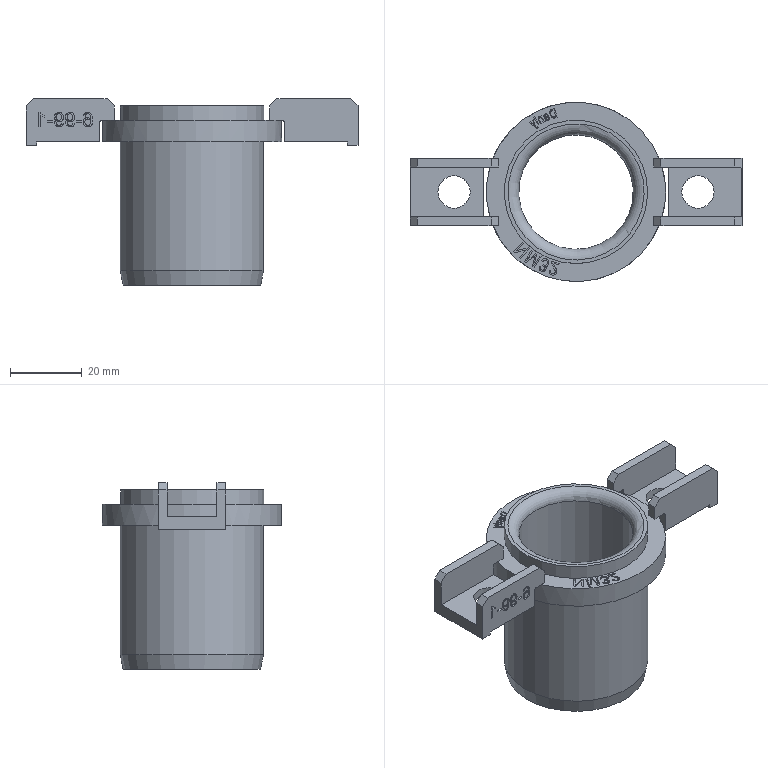Part | STEP file | lll_id4746_x_t | 1 solid | 233 faces | box 92.6 x 50 x 52 mm | volume 30328 mm3 | plane 152 | other 69 | cylinder 10 | torus 1 | cone 1 | commonest cylinder face diameters 1 x4 9 x2 40 x2 32 x1 50 x1